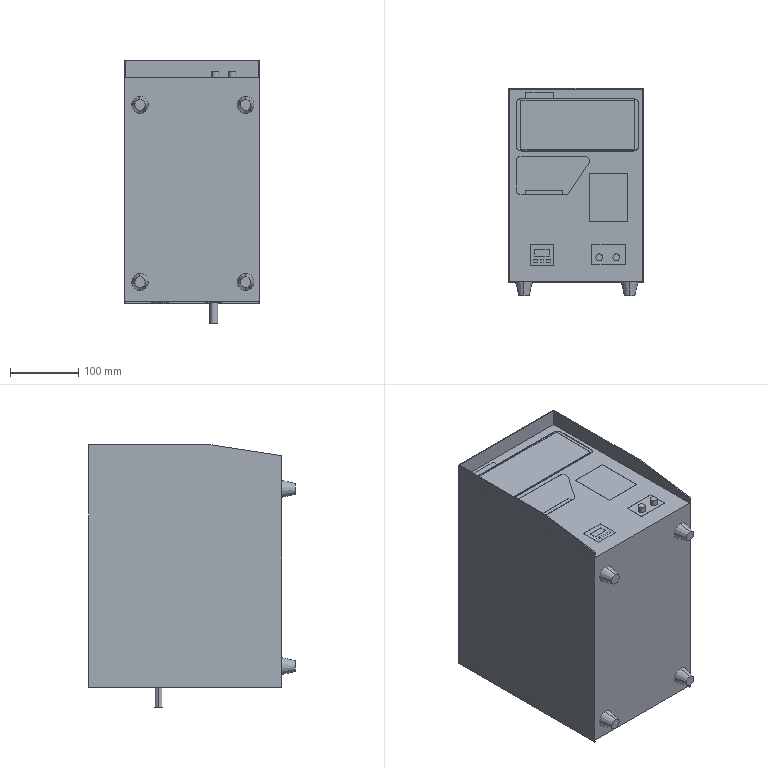Part | STEP file | Cosmo LS-1862 | 5 solids | 125 faces | box 198 x 303.553 x 384.993 mm | volume 18480942 mm3 | plane 95 | cylinder 22 | cone 8 | commonest cylinder face diameters 14 x12 10 x4 11.41 x2 23.57 x2 25.657 x2